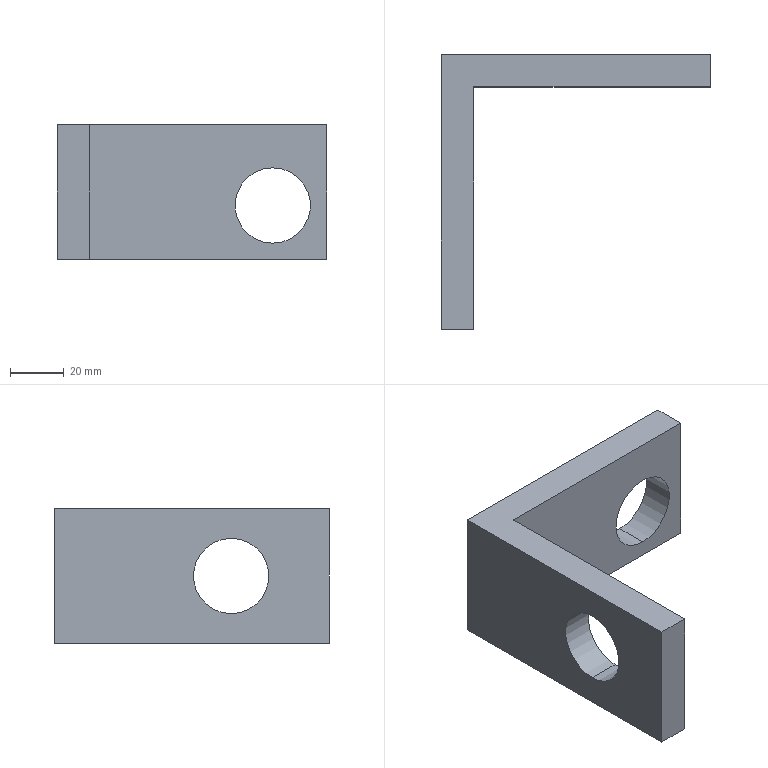Part | SolidWorks | features ICE 3, Extrusion 1, MoveFace 1 | 1 solid | 12 faces | box 100 x 102 x 50 mm | volume 99222 mm3 | plane 8 | cylinder 4 | commonest cylinder face diameters 28 x4
STEP:
#1=CARTESIAN_POINT('',(-80.,-53.54,14.));
#2=VERTEX_POINT('',#1);
#3=CARTESIAN_POINT('',(-80.,-53.54,-14.));
#4=VERTEX_POINT('',#3);
#5=CARTESIAN_POINT('',(-80.,-53.54,0.));
#6=DIRECTION('',(1.,0.,0.));
#7=DIRECTION('',(0.,0.,-1.));
#8=AXIS2_PLACEMENT_3D('',#5,#6,#7);
#9=CIRCLE('',#8,14.);
#10=EDGE_CURVE('',#2,#4,#9,.T.);
#11=ORIENTED_EDGE('',*,*,#10,.F.);
#12=CARTESIAN_POINT('',(-68.,-53.54,14.));
#13=VERTEX_POINT('',#12);
#14=CARTESIAN_POINT('',(-80.,-53.54,14.));
#15=DIRECTION('',(1.,0.,0.));
#16=VECTOR('',#15,1000.);
#17=LINE('',#14,#16);
#18=EDGE_CURVE('',#2,#13,#17,.T.);
#19=ORIENTED_EDGE('',*,*,#18,.T.);
#20=CARTESIAN_POINT('',(-68.,-53.54,-14.));
#21=VERTEX_POINT('',#20);
#22=CARTESIAN_POINT('',(-68.,-53.54,0.));
#23=DIRECTION('',(1.,0.,0.));
#24=DIRECTION('',(0.,0.,-1.));
#25=AXIS2_PLACEMENT_3D('',#22,#23,#24);
#26=CIRCLE('',#25,14.);
#27=EDGE_CURVE('',#13,#21,#26,.T.);
#28=ORIENTED_EDGE('',*,*,#27,.T.);
#29=CARTESIAN_POINT('',(-80.,-53.54,-14.));
#30=DIRECTION('',(1.,0.,0.));
#31=VECTOR('',#30,1000.);
#32=LINE('',#29,#31);
#33=EDGE_CURVE('',#4,#21,#32,.T.);
#34=ORIENTED_EDGE('',*,*,#33,.F.);
#35=EDGE_LOOP('',(#11,#19,#28,#34));
#36=FACE_OUTER_BOUND('',#35,.T.);
#37=CARTESIAN_POINT('',(-80.,-53.54,0.));
#38=DIRECTION('',(1.,0.,0.));
#39=DIRECTION('',(0.,0.,-1.));
#40=AXIS2_PLACEMENT_3D('',#37,#38,#39);
#41=CYLINDRICAL_SURFACE('',#40,14.);
#42=ADVANCED_FACE('',(#36),#41,.F.);
#43=CARTESIAN_POINT('',(0.,0.,-19.));
#44=VERTEX_POINT('',#43);
#45=CARTESIAN_POINT('',(0.,0.,9.));
#46=VERTEX_POINT('',#45);
#47=CARTESIAN_POINT('',(0.,0.,-5.));
#48=DIRECTION('',(0.,1.,0.));
#49=DIRECTION('',(0.,0.,1.));
#50=AXIS2_PLACEMENT_3D('',#47,#48,#49);
#51=CIRCLE('',#50,14.);
#52=EDGE_CURVE('',#44,#46,#51,.T.);
#53=ORIENTED_EDGE('',*,*,#52,.F.);
#54=CARTESIAN_POINT('',(0.,12.,-19.));
#55=VERTEX_POINT('',#54);
#56=CARTESIAN_POINT('',(0.,0.,-19.));
#57=DIRECTION('',(0.,1.,0.));
#58=VECTOR('',#57,1000.);
#59=LINE('',#56,#58);
#60=EDGE_CURVE('',#44,#55,#59,.T.);
#61=ORIENTED_EDGE('',*,*,#60,.T.);
#62=CARTESIAN_POINT('',(0.,12.,9.));
#63=VERTEX_POINT('',#62);
#64=CARTESIAN_POINT('',(0.,12.,-5.));
#65=DIRECTION('',(0.,-1.,0.));
#66=DIRECTION('',(0.,0.,-1.));
#67=AXIS2_PLACEMENT_3D('',#64,#65,#66);
#68=CIRCLE('',#67,14.);
#69=EDGE_CURVE('',#63,#55,#68,.T.);
#70=ORIENTED_EDGE('',*,*,#69,.F.);
#71=CARTESIAN_POINT('',(0.,0.,9.));
#72=DIRECTION('',(0.,1.,0.));
#73=VECTOR('',#72,1000.);
#74=LINE('',#71,#73);
#75=EDGE_CURVE('',#46,#63,#74,.T.);
#76=ORIENTED_EDGE('',*,*,#75,.F.);
#77=EDGE_LOOP('',(#53,#61,#70,#76));
#78=FACE_OUTER_BOUND('',#77,.T.);
#79=CARTESIAN_POINT('',(0.,0.,-5.));
#80=DIRECTION('',(0.,1.,0.));
#81=DIRECTION('',(0.,0.,1.));
#82=AXIS2_PLACEMENT_3D('',#79,#80,#81);
#83=CYLINDRICAL_SURFACE('',#82,14.);
#84=ADVANCED_FACE('',(#78),#83,.F.);
#85=CARTESIAN_POINT('',(0.,0.,-5.));
#86=DIRECTION('',(0.,1.,0.));
#87=DIRECTION('',(0.,0.,1.));
#88=AXIS2_PLACEMENT_3D('',#85,#86,#87);
#89=CIRCLE('',#88,14.);
#90=EDGE_CURVE('',#46,#44,#89,.T.);
#91=ORIENTED_EDGE('',*,*,#90,.T.);
#92=ORIENTED_EDGE('',*,*,#52,.T.);
#93=EDGE_LOOP('',(#91,#92));
#94=FACE_BOUND('',#93,.T.);
#95=CARTESIAN_POINT('',(-68.,0.,25.));
#96=VERTEX_POINT('',#95);
#97=CARTESIAN_POINT('',(20.,0.,25.));
#98=VERTEX_POINT('',#97);
#99=CARTESIAN_POINT('',(-20.,0.,25.));
#100=DIRECTION('',(1.,0.,0.));
#101=VECTOR('',#100,1000.);
#102=LINE('',#99,#101);
#103=EDGE_CURVE('',#96,#98,#102,.T.);
#104=ORIENTED_EDGE('',*,*,#103,.F.);
#105=CARTESIAN_POINT('',(-68.,0.,-25.));
#106=VERTEX_POINT('',#105);
#107=CARTESIAN_POINT('',(-68.,0.,-25.));
#108=DIRECTION('',(0.,0.,-1.));
#109=VECTOR('',#108,1000.);
#110=LINE('',#107,#109);
#111=EDGE_CURVE('',#96,#106,#110,.T.);
#112=ORIENTED_EDGE('',*,*,#111,.T.);
#113=CARTESIAN_POINT('',(20.,0.,-25.));
#114=VERTEX_POINT('',#113);
#115=CARTESIAN_POINT('',(-20.,0.,-25.));
#116=DIRECTION('',(-1.,0.,0.));
#117=VECTOR('',#116,1000.);
#118=LINE('',#115,#117);
#119=EDGE_CURVE('',#114,#106,#118,.T.);
#120=ORIENTED_EDGE('',*,*,#119,.F.);
#121=CARTESIAN_POINT('',(20.,0.,25.));
#122=DIRECTION('',(0.,0.,-1.));
#123=VECTOR('',#122,1000.);
#124=LINE('',#121,#123);
#125=EDGE_CURVE('',#98,#114,#124,.T.);
#126=ORIENTED_EDGE('',*,*,#125,.F.);
#127=EDGE_LOOP('',(#104,#112,#120,#126));
#128=FACE_OUTER_BOUND('',#127,.T.);
#129=CARTESIAN_POINT('',(0.,0.,0.));
#130=DIRECTION('',(0.,-1.,0.));
#131=DIRECTION('',(0.,0.,-1.));
#132=AXIS2_PLACEMENT_3D('',#129,#130,#131);
#133=PLANE('',#132);
#134=ADVANCED_FACE('',(#94,#128),#133,.T.);
#135=ORIENTED_EDGE('',*,*,#125,.T.);
#136=CARTESIAN_POINT('',(20.,12.,-25.));
#137=VERTEX_POINT('',#136);
#138=CARTESIAN_POINT('',(20.,12.,-25.));
#139=DIRECTION('',(0.,-1.,0.));
#140=VECTOR('',#139,1000.);
#141=LINE('',#138,#140);
#142=EDGE_CURVE('',#137,#114,#141,.T.);
#143=ORIENTED_EDGE('',*,*,#142,.F.);
#144=CARTESIAN_POINT('',(20.,12.,25.));
#145=VERTEX_POINT('',#144);
#146=CARTESIAN_POINT('',(20.,12.,25.));
#147=DIRECTION('',(0.,0.,-1.));
#148=VECTOR('',#147,1000.);
#149=LINE('',#146,#148);
#150=EDGE_CURVE('',#145,#137,#149,.T.);
#151=ORIENTED_EDGE('',*,*,#150,.F.);
#152=CARTESIAN_POINT('',(20.,12.,25.));
#153=DIRECTION('',(0.,-1.,0.));
#154=VECTOR('',#153,1000.);
#155=LINE('',#152,#154);
#156=EDGE_CURVE('',#145,#98,#155,.T.);
#157=ORIENTED_EDGE('',*,*,#156,.T.);
#158=EDGE_LOOP('',(#135,#143,#151,#157));
#159=FACE_OUTER_BOUND('',#158,.T.);
#160=CARTESIAN_POINT('',(20.,12.,25.));
#161=DIRECTION('',(-1.,0.,0.));
#162=DIRECTION('',(0.,0.,1.));
#163=AXIS2_PLACEMENT_3D('',#160,#161,#162);
#164=PLANE('',#163);
#165=ADVANCED_FACE('',(#159),#164,.F.);
#166=ORIENTED_EDGE('',*,*,#119,.T.);
#167=CARTESIAN_POINT('',(-68.,-90.,-25.));
#168=VERTEX_POINT('',#167);
#169=CARTESIAN_POINT('',(-68.,-90.,-25.));
#170=DIRECTION('',(0.,1.,0.));
#171=VECTOR('',#170,1000.);
#172=LINE('',#169,#171);
#173=EDGE_CURVE('',#168,#106,#172,.T.);
#174=ORIENTED_EDGE('',*,*,#173,.F.);
#175=CARTESIAN_POINT('',(-80.,-90.,-25.));
#176=VERTEX_POINT('',#175);
#177=CARTESIAN_POINT('',(-80.,-90.,-25.));
#178=DIRECTION('',(-1.,0.,0.));
#179=VECTOR('',#178,1000.);
#180=LINE('',#177,#179);
#181=EDGE_CURVE('',#168,#176,#180,.T.);
#182=ORIENTED_EDGE('',*,*,#181,.T.);
#183=CARTESIAN_POINT('',(-80.,12.,-25.));
#184=VERTEX_POINT('',#183);
#185=CARTESIAN_POINT('',(-80.,12.,-25.));
#186=DIRECTION('',(0.,-1.,0.));
#187=VECTOR('',#186,1000.);
#188=LINE('',#185,#187);
#189=EDGE_CURVE('',#184,#176,#188,.T.);
#190=ORIENTED_EDGE('',*,*,#189,.F.);
#191=CARTESIAN_POINT('',(-20.,12.,-25.));
#192=DIRECTION('',(-1.,0.,0.));
#193=VECTOR('',#192,1000.);
#194=LINE('',#191,#193);
#195=EDGE_CURVE('',#137,#184,#194,.T.);
#196=ORIENTED_EDGE('',*,*,#195,.F.);
#197=ORIENTED_EDGE('',*,*,#142,.T.);
#198=EDGE_LOOP('',(#166,#174,#182,#190,#196,#197));
#199=FACE_OUTER_BOUND('',#198,.T.);
#200=CARTESIAN_POINT('',(-20.,12.,-25.));
#201=DIRECTION('',(0.,0.,1.));
#202=DIRECTION('',(1.,0.,0.));
#203=AXIS2_PLACEMENT_3D('',#200,#201,#202);
#204=PLANE('',#203);
#205=ADVANCED_FACE('',(#199),#204,.F.);
#206=CARTESIAN_POINT('',(-80.,-53.54,0.));
#207=DIRECTION('',(1.,0.,0.));
#208=DIRECTION('',(0.,0.,-1.));
#209=AXIS2_PLACEMENT_3D('',#206,#207,#208);
#210=CIRCLE('',#209,14.);
#211=EDGE_CURVE('',#4,#2,#210,.T.);
#212=ORIENTED_EDGE('',*,*,#211,.T.);
#213=ORIENTED_EDGE('',*,*,#10,.T.);
#214=EDGE_LOOP('',(#212,#213));
#215=FACE_BOUND('',#214,.T.);
#216=ORIENTED_EDGE('',*,*,#189,.T.);
#217=CARTESIAN_POINT('',(-80.,-90.,25.));
#218=VERTEX_POINT('',#217);
#219=CARTESIAN_POINT('',(-80.,-90.,-25.));
#220=DIRECTION('',(0.,0.,1.));
#221=VECTOR('',#220,1000.);
#222=LINE('',#219,#221);
#223=EDGE_CURVE('',#176,#218,#222,.T.);
#224=ORIENTED_EDGE('',*,*,#223,.T.);
#225=CARTESIAN_POINT('',(-80.,12.,25.));
#226=VERTEX_POINT('',#225);
#227=CARTESIAN_POINT('',(-80.,12.,25.));
#228=DIRECTION('',(0.,-1.,0.));
#229=VECTOR('',#228,1000.);
#230=LINE('',#227,#229);
#231=EDGE_CURVE('',#226,#218,#230,.T.);
#232=ORIENTED_EDGE('',*,*,#231,.F.);
#233=CARTESIAN_POINT('',(-80.,12.,25.));
#234=DIRECTION('',(0.,0.,1.));
#235=VECTOR('',#234,1000.);
#236=LINE('',#233,#235);
#237=EDGE_CURVE('',#184,#226,#236,.T.);
#238=ORIENTED_EDGE('',*,*,#237,.F.);
#239=EDGE_LOOP('',(#216,#224,#232,#238));
#240=FACE_OUTER_BOUND('',#239,.T.);
#241=CARTESIAN_POINT('',(-80.,12.,25.));
#242=DIRECTION('',(1.,0.,0.));
#243=DIRECTION('',(0.,0.,-1.));
#244=AXIS2_PLACEMENT_3D('',#241,#242,#243);
#245=PLANE('',#244);
#246=ADVANCED_FACE('',(#215,#240),#245,.F.);
#247=ORIENTED_EDGE('',*,*,#231,.T.);
#248=CARTESIAN_POINT('',(-68.,-90.,25.));
#249=VERTEX_POINT('',#248);
#250=CARTESIAN_POINT('',(-80.,-90.,25.));
#251=DIRECTION('',(1.,0.,0.));
#252=VECTOR('',#251,1000.);
#253=LINE('',#250,#252);
#254=EDGE_CURVE('',#218,#249,#253,.T.);
#255=ORIENTED_EDGE('',*,*,#254,.T.);
#256=CARTESIAN_POINT('',(-68.,-90.,25.));
#257=DIRECTION('',(0.,1.,0.));
#258=VECTOR('',#257,1000.);
#259=LINE('',#256,#258);
#260=EDGE_CURVE('',#249,#96,#259,.T.);
#261=ORIENTED_EDGE('',*,*,#260,.T.);
#262=ORIENTED_EDGE('',*,*,#103,.T.);
#263=ORIENTED_EDGE('',*,*,#156,.F.);
#264=CARTESIAN_POINT('',(-20.,12.,25.));
#265=DIRECTION('',(1.,0.,0.));
#266=VECTOR('',#265,1000.);
#267=LINE('',#264,#266);
#268=EDGE_CURVE('',#226,#145,#267,.T.);
#269=ORIENTED_EDGE('',*,*,#268,.F.);
#270=EDGE_LOOP('',(#247,#255,#261,#262,#263,#269));
#271=FACE_OUTER_BOUND('',#270,.T.);
#272=CARTESIAN_POINT('',(-20.,12.,25.));
#273=DIRECTION('',(0.,0.,-1.));
#274=DIRECTION('',(-1.,0.,0.));
#275=AXIS2_PLACEMENT_3D('',#272,#273,#274);
#276=PLANE('',#275);
#277=ADVANCED_FACE('',(#271),#276,.F.);
#278=ORIENTED_EDGE('',*,*,#69,.T.);
#279=CARTESIAN_POINT('',(0.,12.,-5.));
#280=DIRECTION('',(0.,-1.,0.));
#281=DIRECTION('',(0.,0.,-1.));
#282=AXIS2_PLACEMENT_3D('',#279,#280,#281);
#283=CIRCLE('',#282,14.);
#284=EDGE_CURVE('',#55,#63,#283,.T.);
#285=ORIENTED_EDGE('',*,*,#284,.T.);
#286=EDGE_LOOP('',(#278,#285));
#287=FACE_BOUND('',#286,.T.);
#288=ORIENTED_EDGE('',*,*,#150,.T.);
#289=ORIENTED_EDGE('',*,*,#195,.T.);
#290=ORIENTED_EDGE('',*,*,#237,.T.);
#291=ORIENTED_EDGE('',*,*,#268,.T.);
#292=EDGE_LOOP('',(#288,#289,#290,#291));
#293=FACE_OUTER_BOUND('',#292,.T.);
#294=CARTESIAN_POINT('',(0.,12.,0.));
#295=DIRECTION('',(0.,-1.,0.));
#296=DIRECTION('',(0.,0.,-1.));
#297=AXIS2_PLACEMENT_3D('',#294,#295,#296);
#298=PLANE('',#297);
#299=ADVANCED_FACE('',(#287,#293),#298,.F.);
#300=ORIENTED_EDGE('',*,*,#60,.F.);
#301=ORIENTED_EDGE('',*,*,#90,.F.);
#302=ORIENTED_EDGE('',*,*,#75,.T.);
#303=ORIENTED_EDGE('',*,*,#284,.F.);
#304=EDGE_LOOP('',(#300,#301,#302,#303));
#305=FACE_OUTER_BOUND('',#304,.T.);
#306=CARTESIAN_POINT('',(0.,0.,-5.));
#307=DIRECTION('',(0.,1.,0.));
#308=DIRECTION('',(0.,0.,1.));
#309=AXIS2_PLACEMENT_3D('',#306,#307,#308);
#310=CYLINDRICAL_SURFACE('',#309,14.);
#311=ADVANCED_FACE('',(#305),#310,.F.);
#312=CARTESIAN_POINT('',(-68.,-53.54,0.));
#313=DIRECTION('',(1.,0.,0.));
#314=DIRECTION('',(0.,0.,-1.));
#315=AXIS2_PLACEMENT_3D('',#312,#313,#314);
#316=CIRCLE('',#315,14.);
#317=EDGE_CURVE('',#21,#13,#316,.T.);
#318=ORIENTED_EDGE('',*,*,#317,.F.);
#319=ORIENTED_EDGE('',*,*,#27,.F.);
#320=EDGE_LOOP('',(#318,#319));
#321=FACE_BOUND('',#320,.T.);
#322=ORIENTED_EDGE('',*,*,#111,.F.);
#323=ORIENTED_EDGE('',*,*,#260,.F.);
#324=CARTESIAN_POINT('',(-68.,-90.,-25.));
#325=DIRECTION('',(0.,0.,-1.));
#326=VECTOR('',#325,1000.);
#327=LINE('',#324,#326);
#328=EDGE_CURVE('',#249,#168,#327,.T.);
#329=ORIENTED_EDGE('',*,*,#328,.T.);
#330=ORIENTED_EDGE('',*,*,#173,.T.);
#331=EDGE_LOOP('',(#322,#323,#329,#330));
#332=FACE_OUTER_BOUND('',#331,.T.);
#333=CARTESIAN_POINT('',(-68.,-90.,-25.));
#334=DIRECTION('',(1.,0.,0.));
#335=DIRECTION('',(0.,0.,-1.));
#336=AXIS2_PLACEMENT_3D('',#333,#334,#335);
#337=PLANE('',#336);
#338=ADVANCED_FACE('',(#321,#332),#337,.T.);
#339=ORIENTED_EDGE('',*,*,#223,.F.);
#340=ORIENTED_EDGE('',*,*,#181,.F.);
#341=ORIENTED_EDGE('',*,*,#328,.F.);
#342=ORIENTED_EDGE('',*,*,#254,.F.);
#343=EDGE_LOOP('',(#339,#340,#341,#342));
#344=FACE_OUTER_BOUND('',#343,.T.);
#345=CARTESIAN_POINT('',(0.,-90.,0.));
#346=DIRECTION('',(0.,1.,0.));
#347=DIRECTION('',(0.,0.,1.));
#348=AXIS2_PLACEMENT_3D('',#345,#346,#347);
#349=PLANE('',#348);
#350=ADVANCED_FACE('',(#344),#349,.F.);
#351=ORIENTED_EDGE('',*,*,#18,.F.);
#352=ORIENTED_EDGE('',*,*,#211,.F.);
#353=ORIENTED_EDGE('',*,*,#33,.T.);
#354=ORIENTED_EDGE('',*,*,#317,.T.);
#355=EDGE_LOOP('',(#351,#352,#353,#354));
#356=FACE_OUTER_BOUND('',#355,.T.);
#357=CARTESIAN_POINT('',(-80.,-53.54,0.));
#358=DIRECTION('',(1.,0.,0.));
#359=DIRECTION('',(0.,0.,-1.));
#360=AXIS2_PLACEMENT_3D('',#357,#358,#359);
#361=CYLINDRICAL_SURFACE('',#360,14.);
#362=ADVANCED_FACE('',(#356),#361,.F.);
#363=CLOSED_SHELL('',(#42,#84,#134,#165,#205,#246,#277,#299,#311,#338,#350,#362));
#364=MANIFOLD_SOLID_BREP('',#363);
#365=CARTESIAN_POINT('',(0.,0.,0.));
#366=DIRECTION('',(0.,0.,1.));
#367=DIRECTION('',(1.,0.,0.));
#368=AXIS2_PLACEMENT_3D('',#365,#366,#367);
#369=(LENGTH_UNIT()NAMED_UNIT(*)SI_UNIT(.MILLI.,.METRE.));
#370=UNCERTAINTY_MEASURE_WITH_UNIT(LENGTH_MEASURE(0.00001),#369,'','');
#371=(NAMED_UNIT(*)PLANE_ANGLE_UNIT()SI_UNIT($,.RADIAN.));
#372=(NAMED_UNIT(*)SI_UNIT($,.STERADIAN.)SOLID_ANGLE_UNIT());
#373=(GEOMETRIC_REPRESENTATION_CONTEXT(3)GLOBAL_UNCERTAINTY_ASSIGNED_CONTEXT((#370))GLOBAL_UNIT_ASSIGNED_CONTEXT((#369,#371,#372))REPRESENTATION_CONTEXT('',''));
#374=ADVANCED_BREP_SHAPE_REPRESENTATION('',(#364,#368),#373);